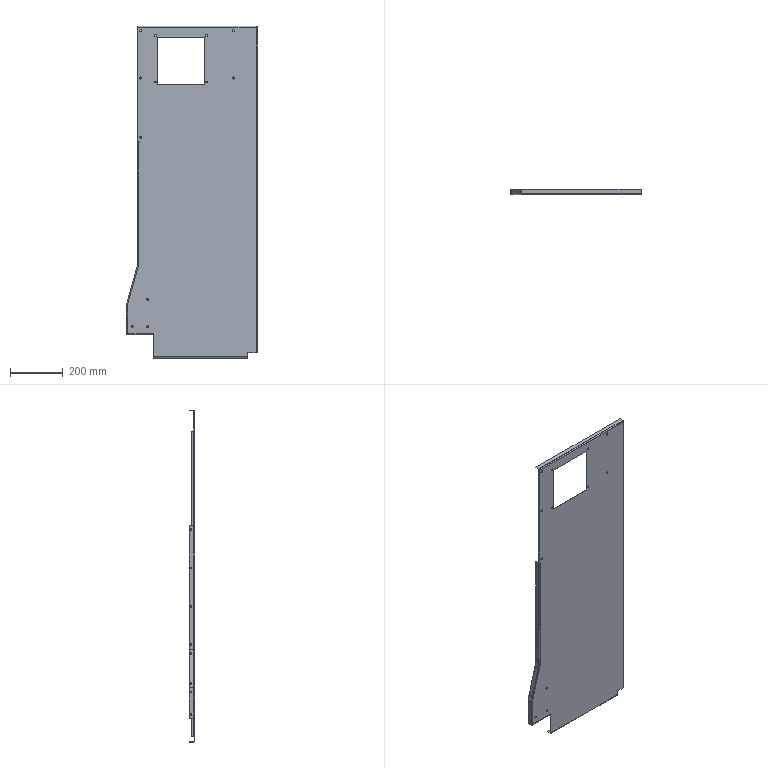Part | NX | features solid 2 | 1 solid | 124 faces | box 496 x 20 x 1263 mm | volume 1163119 mm3 | plane 65 | cylinder 57 | spline 2 | commonest cylinder face diameters 7 x19 8 x17 7.2 x14 4 x7